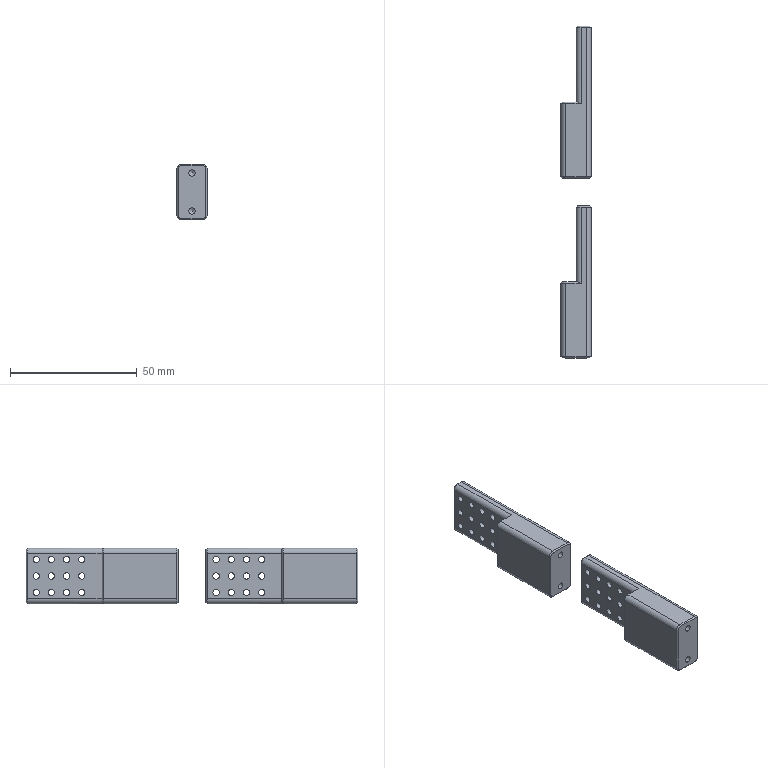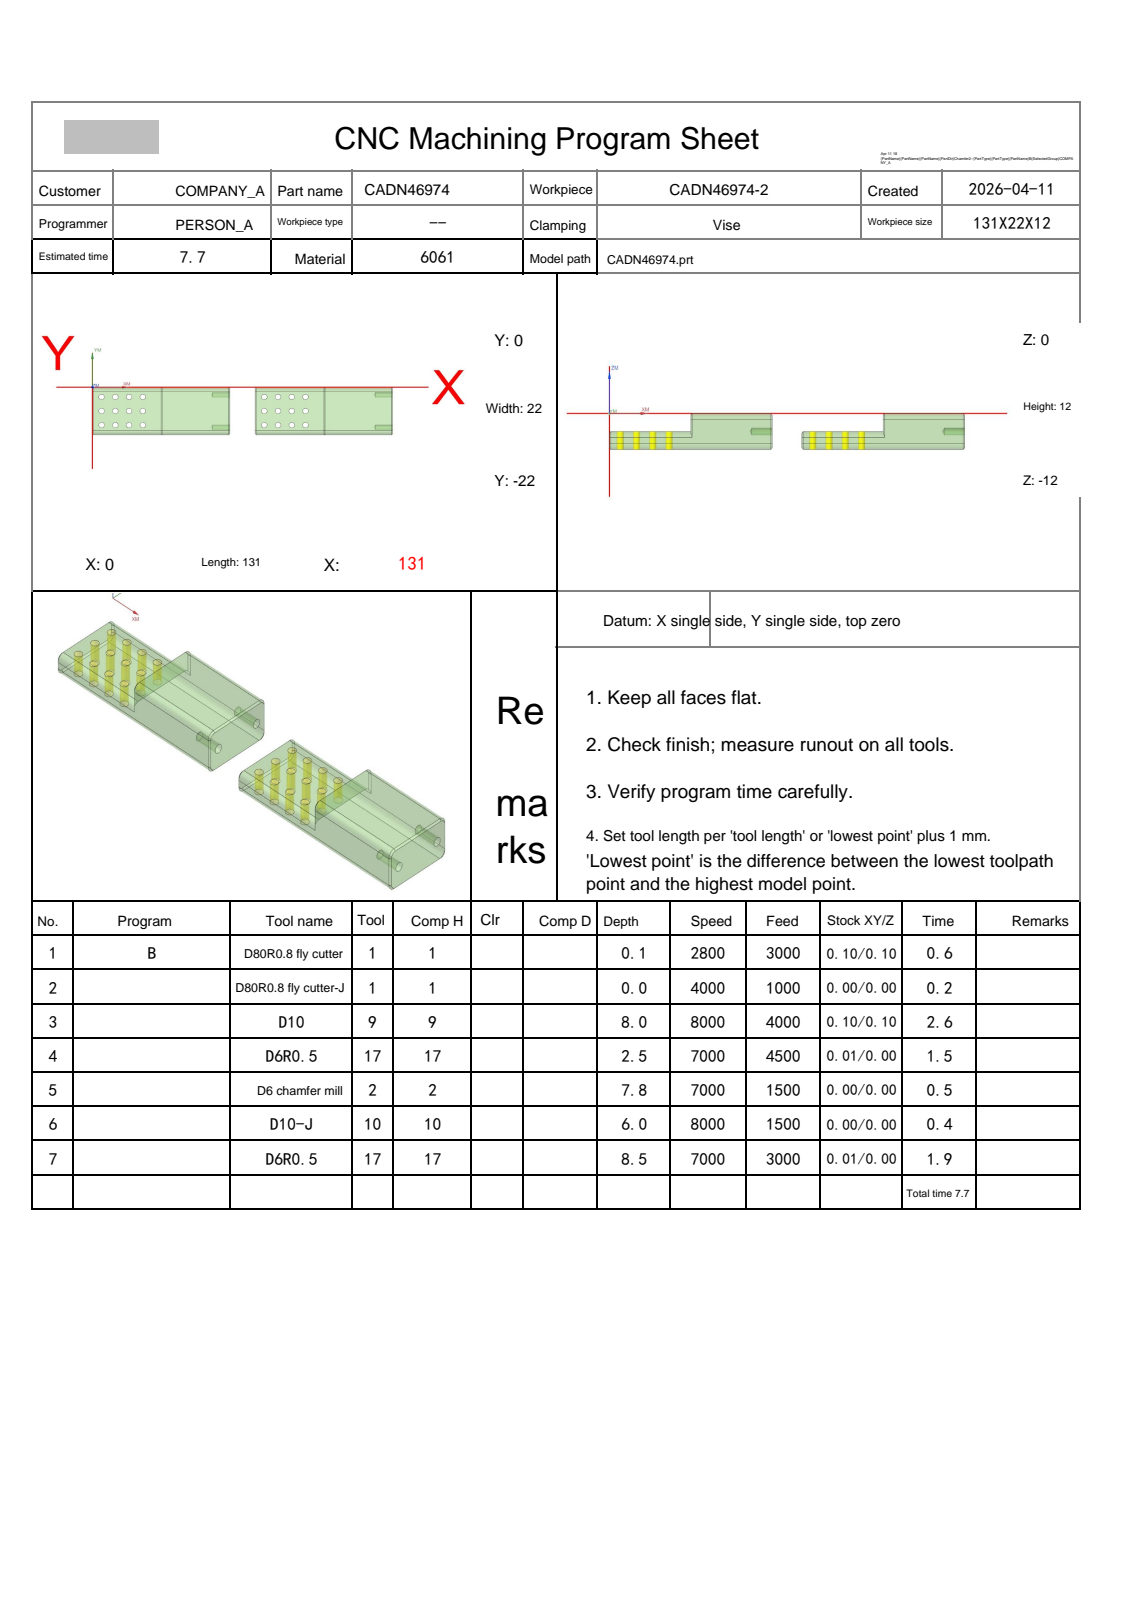NC program | NX | posted by the shop | part box 12 x 131 x 22 mm
Lines 4051 to 5054 of 5054:
N7 T17 M06
(D6R0.5  D=6. R=0.5 H=17 ce=0.01 di=0.00)
G00 G90 G54 X67.696 Y-4.32 M03 S7000
G43 H17 Z12.8
M08
Z-5.509
G01 Z-6.009 F3000.
X67.697
G03 X68.897 Y-3.152 I0.0 J1.2
G01 X68.94 Y-1.554
X68.947 Y-1.515
G02 X71.5 Y.721 I2.671 J-.475
G01 X98.249
X98.303 Y.836 Z-6.021
X71.5
G03 X68.882 Y-1.545 I.079 J-2.716
G01 X68.867 Y-1.686
X68.853 Y-3.152
X68.821 Z-6.03
X68.802 Z-6.038
X68.814 Y-1.686
X68.846 Y-1.453
G02 X71.5 Y.943 I2.751 J-.379
G01 X98.359
X98.417 Y1.046 Z-6.058
X71.5
G03 X68.804 Y-1.433 I.101 J-2.815
G01 X68.774 Y-1.686
X68.761 Y-3.151
X68.734 Z-6.07
X68.717 Z-6.082
X68.727 Y-1.686
X68.774 Y-1.341
G02 X71.5 Y1.147 I2.819 J-.352
G01 X98.48
X98.548 Y1.245 Z-6.111
X71.476
G03 X70.002 Y.772 I0.0 J-2.533
X68.707 Y-1.519 I1.818 J-2.54
G01 X68.692 Y-1.686
X68.681 Y-3.151
X68.658 Z-6.127
X68.641 Z-6.143
X68.653 Y-1.686
X68.687 Y-1.341
G02 X70.366 Y1.088 I3.096 J-.346
X71.5 Y1.342 I1.408 J-3.621
G01 X98.619
X98.696 Y1.437 Z-6.178
X71.5
G03 X69.676 Y.732 I.087 J-2.94
X68.65 Y-1.341 I2.333 J-2.445
G01 X68.615 Y-1.686
X68.605 Y-3.119
X68.565 Y-3.104 Z-6.218
X68.576 Y-1.686
X68.612 Y-1.341
G02 X69.294 Y.41 I3.649 J-.415
X71.5 Y1.53 I2.205 J-1.61
G01 X98.778
X98.865 Y1.622 Z-6.261
X71.5
G03 X68.985 Y.044 I.052 J-2.876
X68.532 Y-1.887 I4.044 J-1.967
G01 X68.522 Y-3.107
X68.476 Y-3.106 Z-6.307
X68.486 Y-1.917
G02 X68.981 Y.136 I4.663 J-.039
X71.5 Y1.711 I2.553 J-1.282
G01 X98.954
X99.041 Y1.798 Z-6.357
X71.5
G03 X69.063 Y.384 I.024 J-2.849
X68.438 Y-1.686 I4.234 J-2.408
G01 X68.425 Y-3.102
X68.372 Y-3.095 Z-6.411
X68.383 Y-1.964
G02 X68.993 Y.377 I4.972 J-.047
X71.5 Y1.883 I2.542 J-1.392
G01 X99.127
X99.209 Y1.966 Z-6.468
X71.5
G03 X68.985 Y.463 I.035 J-2.913
G01 X68.945 Y.384
G03 X68.32 Y-1.877 I4.515 J-2.463
X68.307 Y-2.569 I17.614 J-.691
X68.315 Y-3.107 I17.627 J0.0
G01 X68.255 Y-3.121 Z-6.528
G02 X68.252 Y-2.703 I27.522 J.418
X68.271 Y-1.686 I27.525 J0.0
X69.098 Y.729 I5.271 J-.456
X71.5 Y2.047 I2.422 J-1.567
G01 X99.29
X99.368 Y2.125 Z-6.591
X71.5
G03 X69.038 Y.729 I.025 J-2.914
X68.246 Y-1.341 I4.702 J-2.988
X68.185 Y-2.665 I14.343 J-1.324
X68.192 Y-3.115 I14.404 J0.0
G01 X68.158 Y-3.113 Z-6.624
X68.126 Y-3.112 Z-6.658
G02 X68.119 Y-2.67 I13.767 J.442
X68.183 Y-1.341 I13.774 J0.0
X69.221 Y1.074 I5.503 J-.934
X71.5 Y2.2 I2.296 J-1.778
G01 X99.446
X99.526 Y2.272 Z-6.727
X71.5
G03 X68.985 Y.817 I.025 J-2.944
X68.64 Y.214 I3.192 J-2.228
X68.077 Y-1.789 I4.087 J-2.23
X68.055 Y-2.678 I18.171 J-.889
X68.06 Y-3.129 I18.193 J0.0
G01 X67.994 Y-3.193 Z-6.798
G02 X67.983 Y-2.658 I12.493 J.536
X68.052 Y-1.341 I12.504 J0.0
X68.985 Y.896 I5.325 J-.909
X71.5 Y2.341 I2.537 J-1.505
G01 X99.608
X99.689 Y2.404 Z-6.868
X71.5
G03 X68.985 Y.975 I.025 J-2.972
X67.986 Y-1.341 I4.438 J-3.288
X67.912 Y-2.703 I12.529 J-1.362
X67.918 Y-3.078 I12.603 J0.0
G01 X67.882 Y-3.077 Z-6.904
X67.847 Y-3.076 Z-6.939
X67.858 Y-2.031
G02 X68.369 Y.039 I4.919 J-.118
X69.203 Y1.346 I7.092 J-3.605
X71.5 Y2.463 I2.297 J-1.803
G01 X99.769
X99.85 Y2.517 Z-7.01
X71.5
G03 X70.012 Y2.109 I.021 J-2.993
X68.952 Y1.074 I1.771 J-2.873
X67.853 Y-1.341 I4.64 J-3.569
X67.772 Y-2.748 I12.193 J-1.408
X67.777 Y-3.074 I12.274 J0.0
G01 X67.741 Y-3.073 Z-7.045
X67.706 Y-3.072 Z-7.08
X67.721 Y-2.031
G02 X68.295 Y.117 I4.856 J-.146
X69.261 Y1.529 I7.515 J-4.108
X71.495 Y2.568 I2.234 J-1.883
G01 X99.93
X100.009 Y2.615 Z-7.151
X71.5
G03 X69.625 Y1.935 I0.0 J-2.925
X68.985 Y1.234 I2.259 J-2.704
X68.041 Y-.306 I5.048 J-4.153
X67.653 Y-2.031 I4.112 J-1.831
G01 X67.636 Y-3.07
X67.6 Y-3.069 Z-7.186
X67.565 Y-3.068 Z-7.222
X67.584 Y-2.062
G02 X67.901 Y-.5 I4.409 J-.082
X68.747 Y.985 I5.874 J-2.361
X69.33 Y1.705 I13.013 J-9.954
X71.5 Y2.659 I2.187 J-2.031
G01 X100.089
X100.168 Y2.699 Z-7.293
X71.5
X71.057 Y2.664
G03 X69.33 Y1.752 I.465 J-2.971
G01 X69.048 Y1.419
G03 X68.09 Y.039 I6.386 J-5.459
X67.514 Y-2.031 I3.991 J-2.226
G01 X67.495 Y-3.066
X67.461 Y-2.925 Z-7.328
X67.43 Y-2.784 Z-7.363
Y-2.721
X67.443 Y-2.031
G02 X68.036 Y.039 I4.433 J-.15
X69.307 Y1.764 I8.446 J-4.895
X71.057 Y2.702 I2.203 J-2.007
G01 X71.5 Y2.737
X100.247
X100.325 Y2.771 Z-7.434
X71.5
G03 X69.33 Y1.83 I.012 J-2.999
G01 X69.276 Y1.764
G03 X67.981 Y.039 I7.451 J-6.941
X67.371 Y-2.147 I3.697 J-2.21
G01 X67.361 Y-1.977 Z-7.446
Y-1.806 Z-7.458
X67.37 Y-1.636 Z-7.47
X67.382 Y-1.466 Z-7.482
X67.399 Y-1.297 Z-7.494
X67.432 Y-1.132 Z-7.506
G02 X67.949 Y.076 I3.91 J-.958
X68.64 Y1.072 I12.891 J-8.2
G01 X69.266 Y1.79
G02 X71.494 Y2.804 I2.229 J-1.943
G01 X100.406
X100.491 Y2.836 Z-7.583
X71.5
G03 X69.33 Y1.898 I.01 J-3.003
X67.949 Y.17 I9.585 J-9.075
X67.566 Y-.534 I3.43 J-2.324
G01 X67.596 Y-.41 Z-7.61
X67.631 Y-.289 Z-7.638
X67.679 Y-.173 Z-7.665
G02 X68.012 Y.342 I5.411 J-3.131
X69.33 Y1.932 I12.056 J-8.658
X71.5 Y2.866 I2.185 J-2.087
G01 X100.581
X100.675 Y2.895 Z-7.75
X71.496
G03 X69.381 Y2.009 I0.0 J-2.97
X67.775 Y.088 I10.927 J-10.766
G01 X67.806 Y.188 Z-7.794
X67.852 Y.277 Z-7.838
G02 X68.295 Y.824 I4.457 J-3.156
X69.387 Y2.043 I12.056 J-9.703
X71.5 Y2.921 I2.113 J-2.105
G01 X100.773
X100.873 Y2.944 Z-7.929
X71.5
G03 X69.33 Y2.015 I.011 J-3.022
X67.923 Y.442 I20.738 J-19.98
G01 X67.967 Y.551 Z-8.023
G02 X69.33 Y2.036 I27.889 J-24.238
X71.5 Y2.964 I2.176 J-2.087
G01 X100.977
X101.083 Y2.981 Z-8.12
X71.5
G03 X69.384 Y2.109 I.012 J-3.034
X68.004 Y.637 I32.649 J-31.986
G01 X68.043 Y.718 Z-8.215
G02 X69.37 Y2.109 I51.633 J-47.882
X71.5 Y2.994 I2.145 J-2.159
G01 X101.187
X101.291 Y3.003 Z-8.31
X71.5
G03 X69.364 Y2.109 I.023 J-3.054
X68.065 Y.766 I50.334 J-49.93
G01 X68.079 Y.804 Z-8.405
X68.101 Y.827
X69.33 Y2.081
G02 X71.5 Y3.008 I2.174 J-2.085
G01 X101.396
X101.5 Y3.01
X102.59 Y3.009
X102.601 Y3.01 Z-8.5
X101.5
X101.441
X71.5
G03 X69.472 Y2.223 I0.0 J-3.008
G01 X69.432 Y2.187
X68.086 Y.833
G00 Z12.8
X97.79 Y-24.224
Z-5.509
G01 Z-6.009
G03 X98.352 Y-23.208 I-.638 J1.016
X98.249 Y-22.721 I-1.2 J0.0
G01 X71.612
G02 X68.944 Y-20.459 I0.0 J2.705
G01 X68.92 Y-20.314
X68.897 Y-18.9
X68.853 Z-6.021
X68.867 Y-20.314
X68.882 Y-20.455
G03 X71.5 Y-22.836 I2.697 J.335
G01 X98.303
X98.359 Y-22.943 Z-6.038
X71.5
G02 X68.901 Y-20.754 I.071 J2.721
G01 X68.814 Y-20.314
X68.802 Y-18.9
X68.761 Z-6.058
X68.774 Y-20.314
X68.804 Y-20.567
G03 X71.5 Y-23.046 I2.797 J.336
G01 X98.417
X98.48 Y-23.147 Z-6.082
X71.5
G02 X68.774 Y-20.659 I.092 J2.839
G01 X68.727 Y-20.314
X68.717 Y-18.9
X68.698 Z-6.096
X68.681 Z-6.111
G03 X68.659 Y-19.501 I8.132 J-.601
X68.799 Y-21.004 I8.154 J0.0
X71.5 Y-23.245 I2.807 J.635
G01 X98.548
X98.619 Y-23.342 Z-6.143
X71.499
G02 X69.214 Y-22.073 I0.0 J2.691
X68.651 Y-20.137 I3.162 J1.969
G01 X68.641 Y-18.9
X68.605 Y-18.881 Z-6.178
X68.614 Y-20.14
G03 X68.986 Y-21.797 I4.007 J.029
X71.5 Y-23.437 I2.57 J1.192
G01 X98.696
X98.778 Y-23.53 Z-6.218
X71.5
G02 X69.052 Y-22.04 I.044 J2.828
X68.575 Y-20.174 I3.533 J1.897
G01 X68.565 Y-18.896
X68.522 Y-18.893 Z-6.261
X68.532 Y-20.113
G03 X68.985 Y-22.044 I4.497 J.036
X71.5 Y-23.622 I2.566 J1.299
G01 X98.865
X98.954 Y-23.711 Z-6.307
X71.5
G02 X68.981 Y-22.136 I.035 J2.857
X68.486 Y-20.083 I4.168 J2.093
G01 X68.476 Y-18.894
X68.425 Y-18.898 Z-6.357
Y-19.969
Y-19.971
G03 X69.063 Y-22.384 I4.887 J0.0
X71.5 Y-23.798 I2.461 J1.435
G01 X99.041
X99.127 Y-23.883 Z-6.411
X71.5
G02 X68.993 Y-22.377 I.035 J2.898
X68.383 Y-20.036 I4.361 J2.388
G01 X68.372 Y-18.905
X68.315 Y-18.893 Z-6.468
G03 X68.307 Y-19.429 I17.861 J-.536
X68.321 Y-20.131 I17.869 J0.0
X68.886 Y-22.27 I5.092 J.2
G01 X68.985 Y-22.463
G03 X71.5 Y-23.966 I2.55 J1.41
G01 X99.209
X99.29 Y-24.047 Z-6.528
X71.5
G02 X69.098 Y-22.729 I.019 J2.885
X68.256 Y-19.969 I4.409 J2.853
G01 X68.255 Y-19.624
Y-18.879
X68.192 Y-18.885 Z-6.591
G03 X68.185 Y-19.328 I14.67 J-.443
X68.245 Y-20.659 I14.676 J0.0
X69.038 Y-22.729 I5.499 J.92
X71.5 Y-24.125 I2.487 J1.518
G01 X99.368
X99.446 Y-24.2 Z-6.658
X71.5
G02 X69.221 Y-23.074 I.017 J2.904
X68.183 Y-20.659 I4.47 J3.352
X68.119 Y-19.338 I13.67 J1.321
X68.126 Y-18.915 I13.734 J0.0
G01 X68.092 Y-18.916 Z-6.692
X68.059 Y-18.917 Z-6.727
X68.062 Y-19.96
G03 X68.484 Y-21.897 I4.737 J.019
X69.107 Y-23.006 I6.777 J3.073
X71.497 Y-24.272 I2.391 J1.624
G01 X99.526
X99.608 Y-24.341 Z-6.798
X71.5
G02 X68.985 Y-22.896 I.022 J2.949
G01 X68.872 Y-22.729
G02 X67.993 Y-19.969 I4.345 J2.903
G01 X67.988 Y-19.624
X67.989 Y-18.919
X67.954 Y-18.921 Z-6.833
X67.92 Y-18.922 Z-6.868
G03 X67.912 Y-19.35 I11.773 J-.429
X67.985 Y-20.659 I11.78 J0.0
X68.985 Y-22.975 I5.439 J.976
X71.5 Y-24.404 I2.54 J1.542
G01 X99.689
X99.769 Y-24.463 Z-6.939
X71.499
G02 X69.203 Y-23.346 I0.0 J2.918
X68.369 Y-22.039 I6.287 J4.934
X67.857 Y-19.969 I4.376 J2.181
G01 X67.849 Y-18.924
X67.814 Y-18.925 Z-6.974
X67.779 Y-18.926 Z-7.01
X67.788 Y-19.885
G03 X68.387 Y-22.181 I4.884 J.047
X69.212 Y-23.419 I7.447 J4.071
X71.5 Y-24.517 I2.302 J1.863
G01 X99.85
X99.93 Y-24.568 Z-7.08
X71.496
G02 X69.261 Y-23.529 I0.0 J2.923
X68.295 Y-22.119 I6.587 J5.551
X67.722 Y-19.969 I4.229 J2.279
G01 X67.709 Y-18.928
X67.673 Y-18.929 Z-7.116
X67.639 Y-18.93 Z-7.151
X67.65 Y-19.858
G03 X68.272 Y-22.171 I4.846 J.062
X69.304 Y-23.625 I7.402 J4.162
X71.497 Y-24.615 I2.192 J1.933
G01 X100.009
X100.089 Y-24.659 Z-7.222
X71.5
G02 X69.384 Y-23.764 I.018 J2.991
X68.295 Y-22.305 I7.035 J6.39
X67.653 Y-20.659 I4.306 J2.628
X67.566 Y-19.186 I12.43 J1.474
X67.568 Y-18.932 I12.517 J0.0
G01 X67.533 Y-18.933 Z-7.257
X67.498 Y-18.934 Z-7.293
X67.517 Y-19.969
G03 X68.087 Y-22.039 I4.508 J.128
X69.048 Y-23.419 I7.566 J4.245
G01 X69.33 Y-23.752
G03 X71.057 Y-24.664 I2.185 J2.048
G01 X71.5 Y-24.699
X100.168
X100.247 Y-24.737 Z-7.363
X71.5
X71.057 Y-24.702
G02 X69.414 Y-23.879 I.458 J2.965
X68.03 Y-22.036 I7.263 J6.892
X67.479 Y-20.355 I3.638 J2.124
X67.431 Y-19.442 I8.627 J.913
X67.434 Y-19.206 I8.675 J0.0
G01 X67.419 Y-19.359 Z-7.381
X67.404 Y-19.512 Z-7.399
X67.39 Y-19.666 Z-7.416
X67.377 Y-19.819 Z-7.434
Y-19.869
G03 X67.978 Y-22.039 I4.221 J0.0
X69.371 Y-23.864 I8.832 J5.298
X71.495 Y-24.771 I2.125 J2.034
G01 X100.325
X100.406 Y-24.804 Z-7.506
X71.5
G02 X69.33 Y-23.865 I.012 J3.004
G01 X69.244 Y-23.764
X68.985 Y-23.472
G02 X67.922 Y-22.039 I7.169 J6.433
X67.433 Y-20.88 I3.372 J2.105
G01 X67.452 Y-21.033 Z-7.526
X67.48 Y-21.185 Z-7.545
X67.518 Y-21.333 Z-7.564
X67.567 Y-21.476 Z-7.583
G03 X67.854 Y-22.027 I3.229 J1.336
X69.026 Y-23.56 I9.883 J6.338
G01 X69.314 Y-23.879
G03 X71.5 Y-24.836 I2.192 J2.033
G01 X100.491
X100.581 Y-24.866 Z-7.665
X71.5
G02 X69.394 Y-23.994 I.011 J3.005
X67.949 Y-22.261 I10.563 J10.275
X67.678 Y-21.833 I3.145 J2.291
G01 X67.72 Y-21.966 Z-7.707
X67.774 Y-22.092 Z-7.75
G03 X68.295 Y-22.778 I6.15 J4.133
X69.075 Y-23.686 I8.669 J6.666
G01 X69.297 Y-23.917
X69.33 Y-23.963
G03 X71.5 Y-24.895 I2.186 J2.098
G01 X100.675
X100.773 Y-24.921 Z-7.838
X71.497
G02 X69.394 Y-24.049 I0.0 J2.97
X68.416 Y-22.977 I11.478 J11.457
G01 X67.922 Y-22.384
X67.85 Y-22.282
X67.88 Y-22.367 Z-7.884
X67.92 Y-22.445 Z-7.929
G03 X69.355 Y-24.037 I21.841 J18.229
X71.499 Y-24.944 I2.144 J2.083
G01 X100.873
X100.977 Y-24.964 Z-8.023
X71.5
G02 X69.288 Y-23.994 I.009 J3.026
X68.033 Y-22.633 I35.247 J33.777
G01 X68.021 Y-22.648 Z-8.072
X68.015 Y-22.656 Z-8.12
G03 X69.272 Y-23.994 I44.773 J40.799
X71.5 Y-24.981 I2.254 J2.08
G01 X101.083
X101.187 Y-24.994 Z-8.215
X71.5
G02 X69.371 Y-24.109 I.011 J3.03
X67.998 Y-22.675 I63.179 J61.845
G01 X68.064 Y-22.769 Z-8.31
G03 X69.495 Y-24.238 I55.652 J52.802
X71.5 Y-25.003 I2.027 J2.303
G01 X101.291
X101.454 Y-25.01 Z-8.322
X101.616 Z-8.334
X102.265 Z-8.381
X102.428 Z-8.393
X102.59 Y-25.009 Z-8.405
X101.5 Y-25.01
X101.396 Y-25.008
X71.497
G02 X69.385 Y-24.136 I0.0 J2.994
G01 X69.358 Y-24.109
X68.077 Y-22.807
X68.085 Y-22.834 Z-8.5
X69.361 Y-24.118
G03 X71.503 Y-25.01 I2.143 J2.128
G01 X101.441
X101.5
X102.601
G00 Z12.8
X-3.304 Y-4.406
Z-5.509
G01 Z-6.009
X-3.303
G03 X-2.103 Y-3.208 I0.0 J1.2
G01 X-2.1 Y-1.953
G02 X.5 Y.721 I2.717 J-.042
G01 X27.249
X27.303 Y.836 Z-6.021
X.5
G03 X-2.135 Y-1.869 I.101 J-2.734
G01 X-2.148 Y-3.172
X-2.198 Y-3.133 Z-6.038
X-2.187 Y-1.686
X-2.133 Y-1.341
G02 X.5 Y.943 I2.719 J-.475
G01 X27.359
X27.417 Y1.046 Z-6.058
X.5
G03 X-2.197 Y-1.436 I.097 J-2.811
G01 X-2.226 Y-1.686
X-2.24 Y-3.098
X-2.282 Y-3.14 Z-6.082
X-2.273 Y-1.686
X-2.226 Y-1.341
G02 X.5 Y1.147 I2.832 J-.367
G01 X27.48
X27.548 Y1.245 Z-6.111
X.5
G03 X-2.273 Y-1.341 I.11 J-2.898
G01 X-2.304 Y-1.686
X-2.319 Y-3.109
X-2.342 Y-3.107 Z-6.127
X-2.359 Y-3.106 Z-6.143
G02 X-2.377 Y-2.537 I9.052 J.569
X-2.27 Y-1.15 I9.07 J0.0
X-.716 Y1.045 I2.978 J-.461
X.5 Y1.342 I1.431 J-3.22
G01 X27.619
X27.696 Y1.437 Z-6.178
X.5
G03 X-2.288 Y-.996 I.128 J-2.961
X-2.407 Y-2.597 I10.723 J-1.602
X-2.395 Y-3.103 I10.842 J0.0
G01 X-2.435 Y-3.112 Z-6.218
G02 X-2.447 Y-2.563 I11.872 J.549
X-2.384 Y-1.341 I11.885 J0.0
X-1.51 Y.646 I3.442 J-.33
X.479 Y1.53 I1.989 J-1.794
G01 X27.778
X27.865 Y1.622 Z-6.261
X.5
G03 X-1.804 Y.384 I.038 J-2.834
X-2.436 Y-1.395 I3.35 J-2.191
G01 X-2.466 Y-1.686
X-2.478 Y-3.105
X-2.524 Y-3.104 Z-6.307
X-2.513 Y-1.865
G02 X-1.898 Y.345 I4.419 J-.04
X.498 Y1.711 I2.395 J-1.417
G01 X27.954
X28.041 Y1.798 Z-6.357
X.5
G03 X-1.942 Y.384 I.04 J-2.886
X-2.567 Y-1.807 I4.238 J-2.393
X-2.582 Y-2.566 I18.343 J-.759
X-2.575 Y-3.102 I18.359 J0.0
G01 X-2.628 Y-3.101 Z-6.411
Y-2.031
G02 X-1.996 Y.384 I5.041 J-.03
X.5 Y1.883 I2.52 J-1.368
G01 X28.127
X28.209 Y1.966 Z-6.468
X.5
G03 X-1.754 Y.851 I.029 J-2.893
X-2.685 Y-2.031 I4.115 J-2.921
G01 Y-3.099
X-2.745 Y-3.097 Z-6.528
G02 X-2.758 Y-2.553 I11.601 J.544
X-2.694 Y-1.341 I11.614 J0.0
X-1.908 Y.729 I5.479 J-.898
X.5 Y2.047 I2.433 J-1.588
G01 X28.29
X28.368 Y2.125 Z-6.591
X.5
G03 X-1.963 Y.729 I.025 J-2.915
X-2.757 Y-1.341 I4.764 J-3.015
X-2.821 Y-2.565 I11.756 J-1.225
X-2.808 Y-3.103 I11.819 J0.0
G01 X-2.874 Y-3.157 Z-6.658
G02 X-2.881 Y-2.681 I14.736 J.476
X-2.82 Y-1.341 I14.743 J0.0
X-2.014 Y.729 I5.464 J-.936
G01 X-1.781 Y1.074
G02 X.5 Y2.2 I2.302 J-1.791
G01 X28.446
X28.526 Y2.272 Z-6.727
X.497
G03 X-1.896 Y.989 I0.0 J-2.872
G01 X-2.068 Y.729
G03 X-2.884 Y-1.341 I4.491 J-2.965
X-2.947 Y-2.636 I13.161 J-1.296
X-2.936 Y-3.186 I13.224 J0.0
G01 X-3.008 Y-3.155 Z-6.798
G02 X-3.017 Y-2.666 I12.847 J.489
X-2.982 Y-1.722 I12.856 J0.0
X-2.1 Y.766 I4.982 J-.367
X.5 Y2.341 I2.651 J-1.443
G01 X28.608
X28.689 Y2.404 Z-6.868
X.5
G03 X-1.677 Y1.419 I.013 J-2.925
X-2.176 Y.729 I3.261 J-2.888
X-3.072 Y-2.031 I4.113 J-2.86
G01 X-3.073 Y-3.238
X-3.117 Y-3.157 Z-6.904
X-3.153 Y-3.076 Z-6.939
X-3.14 Y-2.068
G02 X-2.358 Y.531 I4.919 J-.063
G01 X-2.23 Y.729
G02 X-1.807 Y1.334 I6.303 J-3.962
X.499 Y2.463 I2.305 J-1.791
G01 X28.769
X28.85 Y2.517 Z-7.01
X.5
G03 X-1.786 Y1.419 I.021 J-2.972
X-2.502 Y.384 I8.041 J-6.334
X-3.209 Y-2.031 I4.266 J-2.559
G01 X-3.223 Y-3.074
X-3.259 Y-3.073 Z-7.045
X-3.294 Y-3.072 Z-7.08
X-3.278 Y-2.031
G02 X-2.553 Y.384 I4.925 J-.163
X-1.749 Y1.516 I7.582 J-4.533
X.5 Y2.568 I2.249 J-1.88
G01 X28.93
X29.009 Y2.615 Z-7.151
X.499
G03 X-1.694 Y1.628 I0.0 J-2.929
X-2.792 Y.056 I6.242 J-5.531
X-3.348 Y-2.031 I4.272 J-2.255
G01 X-3.364 Y-3.07
X-3.4 Y-3.069 Z-7.186
X-3.435 Y-3.068 Z-7.222
X-3.417 Y-2.031
G02 X-2.792 Y.144 I4.61 J-.148
G01 X-2.445 Y.729
G02 X-1.754 Y1.613 I14.067 J-10.289
X.5 Y2.659 I2.278 J-1.957
G01 X29.089
X29.168 Y2.699 Z-7.293
X.5
G03 X-1.953 Y1.419 I.042 J-3.072
X-2.627 Y.501 I5.221 J-4.538
G01 X-2.821 Y.185
G03 X-3.488 Y-2.094 I3.845 J-2.361
G01 X-3.505 Y-3.066
X-3.539 Y-2.925 Z-7.328
X-3.57 Y-2.784 Z-7.363
Y-2.721
X-3.557 Y-2.031
G02 X-2.965 Y.039 I4.462 J-.157
X-1.754 Y1.693 I8.343 J-4.837
G01 X-1.695 Y1.764
G02 X-.024 Y2.688 I2.21 J-2.023
G01 X.5 Y2.737
X29.247
X29.325 Y2.771 Z-7.434
X.5
G03 X-1.729 Y1.764 I.016 J-3.005
G01 X-1.754 Y1.734
G03 X-2.961 Y.138 I8.021 J-7.324
X-3.629 Y-2.148 I3.772 J-2.341
G01 X-3.639 Y-1.978 Z-7.446
Y-1.807 Z-7.458
X-3.63 Y-1.636 Z-7.47
X-3.618 Y-1.466 Z-7.482
X-3.601 Y-1.297 Z-7.494
X-3.567 Y-1.133 Z-7.506
G02 X-3.075 Y.039 I3.965 J-.977
X-2.359 Y1.074 I14.879 J-9.528
G01 X-1.762 Y1.764
G02 X.5 Y2.804 I2.278 J-1.974
G01 X29.406
X29.491 Y2.836 Z-7.583
X.5
G03 X-1.657 Y1.911 I0.0 J-2.977
X-3.134 Y.039 I9.327 J-8.878
X-3.435 Y-.535 I3.141 J-2.015
G01 X-3.405 Y-.411 Z-7.61
X-3.369 Y-.289 Z-7.638
X-3.318 Y-.175 Z-7.665
G02 X-3.018 Y.3 I4.338 J-2.411
X-1.643 Y1.956 I12.062 J-8.621
X.496 Y2.866 I2.139 J-2.057
G01 X29.581
X29.675 Y2.895 Z-7.75
X.499
G03 X-1.617 Y2.008 I0.0 J-2.969
X-3.225 Y.091 I11.266 J-11.082
G01 X-3.189 Y.194 Z-7.794
X-3.144 Y.291 Z-7.838
G02 X-1.637 Y2.021 I16.22 J-12.61
X.498 Y2.921 I2.135 J-2.081
G01 X29.773
X29.873 Y2.944 Z-7.929
X.499
G03 X-1.657 Y2.023 I0.0 J-2.982
G01 X-2.234 Y1.419
X-3.09 Y.43
X-3.05 Y.527 Z-8.023
G02 X-1.598 Y2.109 I24.723 J-21.228
X.5 Y2.964 I2.106 J-2.167
G01 X29.977
X30.083 Y2.981 Z-8.12
X.5
X.456 Y2.975
G03 X-1.616 Y2.109 I.037 J-3.001
X-3.006 Y.625 I31.425 J-30.835
G01 X-2.958 Y.716 Z-8.215
G02 X-1.627 Y2.109 I35.655 J-32.728
X.5 Y2.994 I2.137 J-2.14
G01 X30.187
X30.291 Y3.003 Z-8.31
X.5
X.498
G03 X-1.634 Y2.109 I0.0 J-2.99
X-2.932 Y.771 I46.94 J-46.804
G01 X-2.922 Y.804 Z-8.405
G02 X-1.641 Y2.109 I72.22 J-69.615
X.5 Y3.008 I2.143 J-2.105
G01 X30.396
X30.497 Y3.01
X31.6
Z-8.5
X30.497
X30.437
X.5
G03 X-1.635 Y2.122 I0.0 J-3.01
G01 X-2.677 Y1.074
X-2.915 Y.833
G00 Z12.8
X26.79 Y-24.224
Z-5.509
G01 Z-6.009
G03 X27.352 Y-23.208 I-.638 J1.016
X27.249 Y-22.721 I-1.2 J0.0
G01 X.5
G02 X-2.056 Y-20.434 I.096 J2.68
G01 X-2.074 Y-20.314
X-2.103 Y-18.9
X-2.148 Z-6.021
X-2.135 Y-20.131
G03 X.5 Y-22.836 I2.735 J.029
G01 X27.303
X27.359 Y-22.943 Z-6.038
X.5
G02 X-2.133 Y-20.659 I.086 J2.759
G01 X-2.187 Y-20.314
X-2.198 Y-18.9
X-2.223 Z-6.048
X-2.24 Z-6.058
X-2.226 Y-20.314
X-2.197 Y-20.564
G03 X.5 Y-23.046 I2.793 J.329
G01 X27.417
X27.48 Y-23.147 Z-6.082
X.5
G02 X-2.226 Y-20.659 I.105 J2.853
G01 X-2.273 Y-20.314
X-2.283 Y-18.9
X-2.305 Z-6.096
X-2.319 Z-6.111
X-2.304 Y-20.314
X-2.273 Y-20.659
G03 X.5 Y-23.245 I2.883 J.312
G01 X27.548
X27.619 Y-23.342 Z-6.143
X.498
G02 X-1.212 Y-22.709 I0.0 J2.627
X-2.306 Y-20.659 I2.085 J2.43
X-2.372 Y-19.44 I11.32 J1.219
X-2.359 Y-18.9 I11.386 J0.0
G01 X-2.395 Y-18.897 Z-6.178
G03 X-2.412 Y-19.461 I9.683 J-.564
X-2.288 Y-21.004 I9.699 J0.0
X.5 Y-23.437 I2.916 J.528
G01 X27.696
X27.778 Y-23.53 Z-6.218
X.5
G02 X-1.952 Y-22.039 I.049 J2.841
X-2.384 Y-20.659 I3.347 J1.807
X-2.448 Y-19.445 I11.549 J1.215
X-2.435 Y-18.888 I11.613 J0.0
G01 X-2.478 Y-18.895 Z-6.261
X-2.466 Y-20.314
X-2.446 Y-20.502
G03 X-2.008 Y-22.039 I4.196 J.365
X.5 Y-23.622 I2.551 J1.265
G01 X27.865
X27.954 Y-23.711 Z-6.307
X.498
G02 X-1.909 Y-22.325 I0.0 J2.782
X-2.512 Y-20.314 I3.905 J2.266
G01 X-2.524 Y-18.896
X-2.575 Y-18.898 Z-6.357
Y-18.934
X-2.563 Y-20.083
G03 X-1.942 Y-22.384 I4.741 J.046
X.5 Y-23.798 I2.483 J1.472
G01 X28.041
X28.127 Y-23.883 Z-6.411
X.5
G02 X-1.996 Y-22.384 I.024 J2.867
X-2.628 Y-19.969 I4.408 J2.444
G01 Y-18.899
X-2.685 Y-18.901 Z-6.468
Y-19.969
G03 X-1.754 Y-22.851 I5.046 J.039
X.5 Y-23.966 I2.283 J1.778
G01 X28.209
X28.29 Y-24.047 Z-6.528
X.5
G02 X-1.908 Y-22.729 I.026 J2.905
X-2.694 Y-20.659 I4.692 J2.968
X-2.758 Y-19.45 I11.43 J1.209
X-2.745 Y-18.903 I11.494 J0.0
G01 X-2.808 Y-18.897 Z-6.591
G03 X-2.821 Y-19.441 I11.61 J-.543
X-2.757 Y-20.659 I11.623 J0.0
X-1.963 Y-22.729 I5.556 J.944
X.5 Y-24.125 I2.488 J1.52
G01 X28.368
X28.446 Y-24.2 Z-6.658
X.5
G02 X-1.781 Y-23.074 I.021 J2.916
G01 X-1.954 Y-22.818
G02 X-2.821 Y-20.659 I4.551 J3.079
X-2.881 Y-19.348 I14.248 J1.311
X-2.874 Y-18.915 I14.308 J0.0
G01 X-2.908 Y-18.916 Z-6.692
X-2.94 Y-18.917 Z-6.727
G03 X-2.948 Y-19.373 I12.921 J-.456
X-2.884 Y-20.659 I12.929 J0.0
X-2.068 Y-22.729 I5.312 J.898
G01 X-1.839 Y-23.074
G03 X.5 Y-24.272 I2.356 J1.718
G01 X28.526
X28.608 Y-24.341 Z-6.798
X.5
G02 X-2.1 Y-22.766 I.051 J3.018
X-2.949 Y-20.659 I4.391 J2.995
X-3.018 Y-19.364 I12.179 J1.295
X-3.01 Y-18.919 I12.248 J0.0
G01 X-3.046 Y-18.92 Z-6.833
X-3.08 Y-18.921 Z-6.868
X-3.074 Y-20.002
G03 X-2.712 Y-21.728 I4.423 J.026
X-1.799 Y-23.277 I6.591 J2.843
X.498 Y-24.404 I2.297 J1.777
G01 X28.689
X28.769 Y-24.463 Z-6.939
X.5
G02 X-1.754 Y-23.401 I.023 J2.973
G01 X-1.999 Y-23.074
G02 X-2.758 Y-21.762 I5.565 J4.093
X-3.126 Y-20.252 I4.076 J1.792
X-3.156 Y-19.307 I14.861 J.945
X-3.151 Y-18.924 I14.891 J0.0
G01 X-3.186 Y-18.925 Z-6.974
X-3.221 Y-18.926 Z-7.01
X-3.21 Y-19.969
G03 X-2.686 Y-22.039 I4.784 J.11
X-1.786 Y-23.419 I7.275 J3.763
X.5 Y-24.517 I2.307 J1.874
G01 X28.85
X28.93 Y-24.568 Z-7.08
X.497
G02 X-1.732 Y-23.536 I0.0 J2.924
X-2.746 Y-22.039 I6.373 J5.407
X-3.279 Y-19.969 I4.273 J2.204
G01 X-3.291 Y-18.928
X-3.327 Y-18.929 Z-7.116
X-3.361 Y-18.93 Z-7.151
X-3.347 Y-19.969
G03 X-2.792 Y-22.058 I4.75 J.143
X-1.694 Y-23.628 I7.413 J4.018
X.497 Y-24.615 I2.19 J1.938
G01 X29.009
X29.089 Y-24.659 Z-7.222
X.5
G02 X-1.754 Y-23.613 I.023 J3.001
X-2.254 Y-22.985 I13.441 J11.225
X-3.017 Y-21.708 I5.316 J4.041
X-3.415 Y-19.969 I4.051 J1.842
G01 X-3.432 Y-18.932
X-3.467 Y-18.933 Z-7.257
X-3.502 Y-18.934 Z-7.293
X-3.484 Y-19.94
G03 X-2.83 Y-22.176 I4.424 J.081
G01 X-2.792 Y-22.236
G03 X-1.953 Y-23.419 I6.632 J3.814
G01 X-1.659 Y-23.764
G03 X.5 Y-24.699 I2.195 J2.108
G01 X29.168
X29.247 Y-24.737 Z-7.363
X.5
G02 X-.697 Y-24.48 I.048 J3.148
X-1.627 Y-23.83 I1.111 J2.579
X-2.972 Y-22.032 I7.101 J6.713
X-3.521 Y-20.352 I3.643 J2.12
X-3.569 Y-19.44 I8.69 J.912
X-3.566 Y-19.206 I8.738 J0.0
G01 X-3.581 Y-19.359 Z-7.381
X-3.596 Y-19.512 Z-7.399
X-3.61 Y-19.664 Z-7.416
X-3.623 Y-19.817 Z-7.434
Y-19.869
G03 X-3.023 Y-22.039 I4.222 J0.0
X-2.024 Y-23.419 I7.974 J4.72
G01 X-1.754 Y-23.734
X-1.729 Y-23.764
G03 X.5 Y-24.771 I2.245 J1.999
G01 X29.325
X29.406 Y-24.804 Z-7.506
X.5
G02 X-1.762 Y-23.764 I.016 J3.015
G01 X-2.359 Y-23.074
G02 X-3.079 Y-22.039 I13.331 J10.034
X-3.567 Y-20.881 I3.432 J2.128
G01 X-3.548 Y-21.033 Z-7.526
X-3.52 Y-21.184 Z-7.545
X-3.483 Y-21.331 Z-7.564
X-3.435 Y-21.474 Z-7.583
G03 X-3.138 Y-22.039 I3.342 J1.397
X-1.754 Y-23.808 I10.904 J7.105
G01 X-1.45 Y-24.109
G03 X.5 Y-24.836 I1.966 J2.297
G01 X29.491
X29.581 Y-24.866 Z-7.665
X.498
G02 X-1.647 Y-23.951 I0.0 J2.971
X-3.138 Y-22.137 I11.109 J10.648
G01 X-3.319 Y-21.832
X-3.279 Y-21.968 Z-7.707
X-3.226 Y-22.096 Z-7.75
G03 X-1.476 Y-24.148 I12.886 J9.22
X.5 Y-24.895 I1.992 J2.281
G01 X29.675
X29.773 Y-24.921 Z-7.838
X.498
G02 X-1.662 Y-23.991 I0.0 J2.973
G01 X-1.994 Y-23.64
G02 X-3.146 Y-22.294 I12.975 J12.273
G01 X-3.071 Y-22.43 Z-7.884
X-2.987 Y-22.557 Z-7.929
G03 X-1.639 Y-24.043 I21.385 J18.038
X.498 Y-24.944 I2.137 J2.082
G01 X29.873
X29.977 Y-24.964 Z-8.023
X.5
G02 X-1.65 Y-24.057 I0.0 J3.
X-3.01 Y-22.58 I26.408 J25.703
G01 X-3.023 Y-22.597 Z-8.072
X-3.029 Y-22.606 Z-8.12
G03 X-1.617 Y-24.109 I39.446 J35.652
X.5 Y-24.981 I2.124 J2.152
G01 X30.083
X30.187 Y-24.994 Z-8.215
X.5
G02 X-1.627 Y-24.109 I.007 J3.015
X-3.045 Y-22.623 I39.343 J38.966
G01 X-2.99 Y-22.699 Z-8.262
X-2.934 Y-22.774 Z-8.31
G03 X-1.754 Y-23.987 I82.914 J79.481
G01 X-1.634 Y-24.109
G03 X.5 Y-25.003 I2.15 J2.138
G01 X30.291
X30.455 Y-25.01 Z-8.322
X30.618 Z-8.334
X31.436 Z-8.393
X31.6 Z-8.405
X30.497
X30.396 Y-25.008
X.5
G02 X-1.642 Y-24.109 I.006 J3.015
G01 X-2.923 Y-22.807
X-2.915 Y-22.835 Z-8.5
X-1.754 Y-24.003
X-1.62 Y-24.136
G03 X.498 Y-25.01 I2.119 J2.13
G01 X30.437
X30.497
X31.6
G00 Z12.8
M05
M09
G91 G28 Z0.0
G91 G28 Y0.0
M30
%